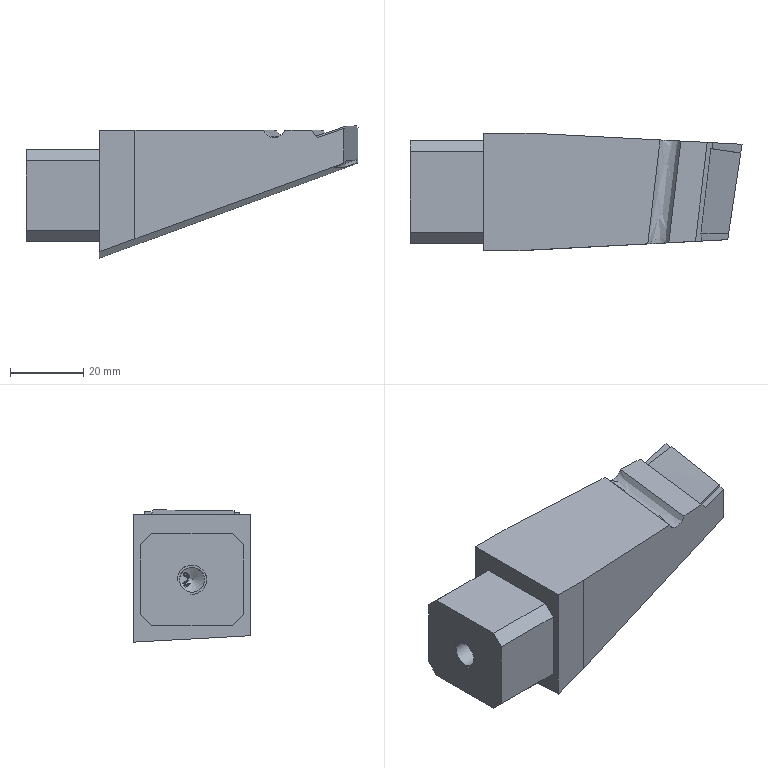Part | STEP file | P011002S003-003 | 1 solid | 64 faces | box 90.488 x 32 x 36.044 mm | volume 56970 mm3 | plane 34 | other 11 | spline 9 | cone 7 | cylinder 3 | commonest cylinder face diameters 6.8 x1 7.973 x1 8 x1